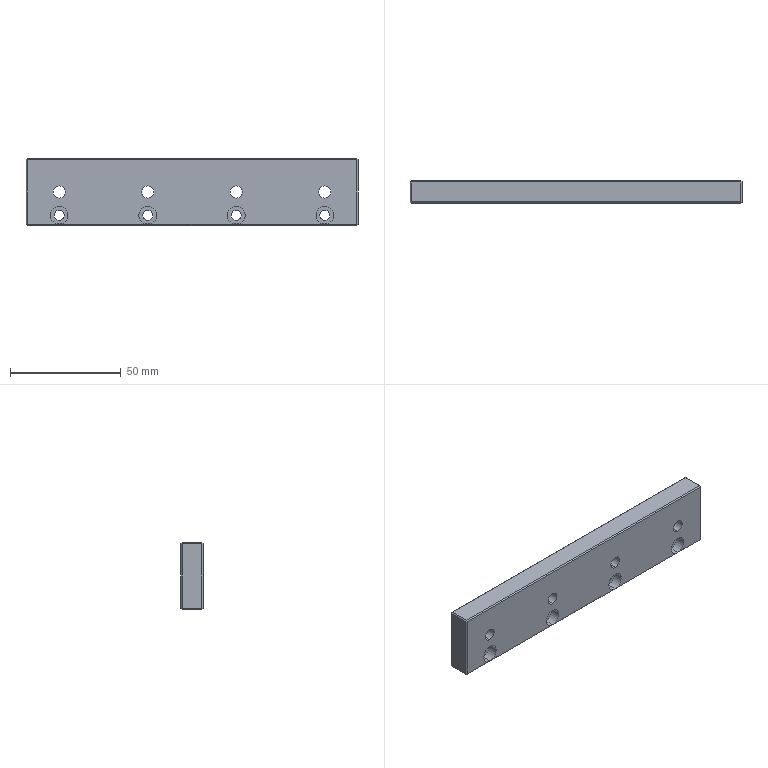Part | STEP file | BPSP-11-003Unloading Support Plate2_Default | 1 solid | 66 faces | box 150 x 10 x 30 mm | volume 41531 mm3 | plane 34 | cylinder 32 | commonest cylinder face diameters 4.5 x8 5.5 x8 8 x8 10 x8